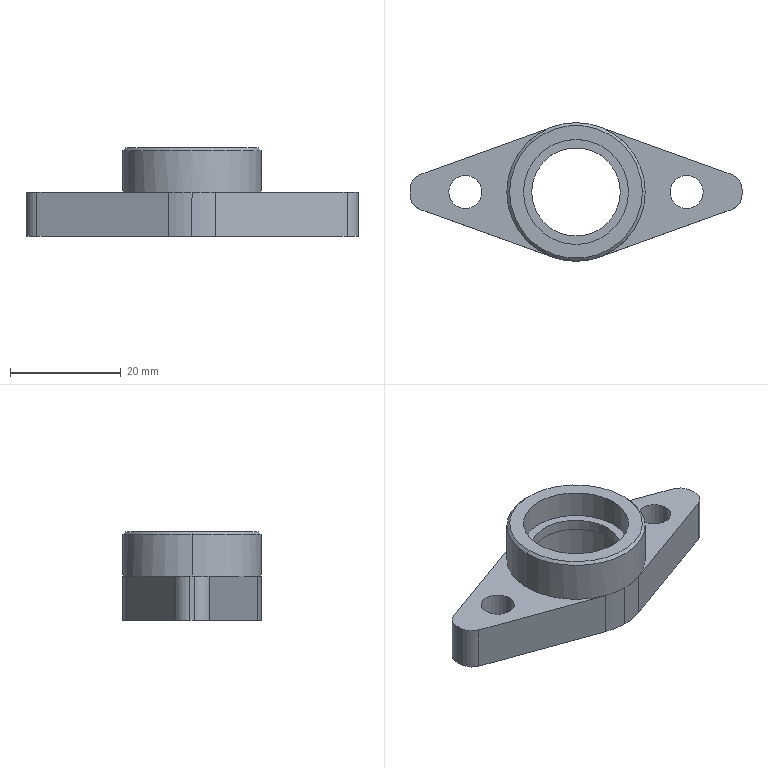Part | SolidWorks | features ICE 5, Fillet 2, MirrorPattern 2, Chamfer 1, Extrusion 1, HoleWzd 1 | 1 solid | 34 faces | box 60 x 25 x 16 mm | volume 6607 mm3 | cylinder 20 | plane 12 | cone 2 | commonest cylinder face diameters 6 x8 25 x6 19 x4 16 x2
STEP:
#1=CARTESIAN_POINT('',(-9.5,12.5,11.));
#2=VERTEX_POINT('',#1);
#3=CARTESIAN_POINT('',(9.5,12.5,11.));
#4=VERTEX_POINT('',#3);
#5=CARTESIAN_POINT('',(0.,12.5,11.));
#6=DIRECTION('',(0.,0.,1.));
#7=DIRECTION('',(1.,0.,0.));
#8=AXIS2_PLACEMENT_3D('',#5,#6,#7);
#9=CIRCLE('',#8,9.5);
#10=EDGE_CURVE('',#2,#4,#9,.T.);
#11=ORIENTED_EDGE('',*,*,#10,.F.);
#12=CARTESIAN_POINT('',(-9.5,12.5,16.));
#13=VERTEX_POINT('',#12);
#14=CARTESIAN_POINT('',(-9.5,12.5,11.));
#15=DIRECTION('',(0.,0.,1.));
#16=VECTOR('',#15,1000.);
#17=LINE('',#14,#16);
#18=EDGE_CURVE('',#2,#13,#17,.T.);
#19=ORIENTED_EDGE('',*,*,#18,.T.);
#20=CARTESIAN_POINT('',(9.5,12.5,16.));
#21=VERTEX_POINT('',#20);
#22=CARTESIAN_POINT('',(0.,12.5,16.));
#23=DIRECTION('',(0.,0.,1.));
#24=DIRECTION('',(1.,0.,0.));
#25=AXIS2_PLACEMENT_3D('',#22,#23,#24);
#26=CIRCLE('',#25,9.5);
#27=EDGE_CURVE('',#13,#21,#26,.T.);
#28=ORIENTED_EDGE('',*,*,#27,.T.);
#29=CARTESIAN_POINT('',(9.5,12.5,11.));
#30=DIRECTION('',(0.,0.,1.));
#31=VECTOR('',#30,1000.);
#32=LINE('',#29,#31);
#33=EDGE_CURVE('',#4,#21,#32,.T.);
#34=ORIENTED_EDGE('',*,*,#33,.F.);
#35=EDGE_LOOP('',(#11,#19,#28,#34));
#36=FACE_OUTER_BOUND('',#35,.T.);
#37=CARTESIAN_POINT('',(0.,12.5,11.));
#38=DIRECTION('',(0.,0.,1.));
#39=DIRECTION('',(1.,0.,0.));
#40=AXIS2_PLACEMENT_3D('',#37,#38,#39);
#41=CYLINDRICAL_SURFACE('',#40,9.5);
#42=ADVANCED_FACE('',(#36),#41,.F.);
#43=CARTESIAN_POINT('',(12.,12.5,16.));
#44=VERTEX_POINT('',#43);
#45=CARTESIAN_POINT('',(-12.,12.5,16.));
#46=VERTEX_POINT('',#45);
#47=CARTESIAN_POINT('',(0.,12.5,16.));
#48=DIRECTION('',(0.,0.,1.));
#49=DIRECTION('',(1.,0.,0.));
#50=AXIS2_PLACEMENT_3D('',#47,#48,#49);
#51=CIRCLE('',#50,12.);
#52=EDGE_CURVE('',#44,#46,#51,.T.);
#53=ORIENTED_EDGE('',*,*,#52,.F.);
#54=CARTESIAN_POINT('',(12.5,12.5,15.5));
#55=VERTEX_POINT('',#54);
#56=CARTESIAN_POINT('',(12.,12.5,16.));
#57=DIRECTION('',(0.7071,0.,-0.7071));
#58=VECTOR('',#57,1000.);
#59=LINE('',#56,#58);
#60=EDGE_CURVE('',#44,#55,#59,.T.);
#61=ORIENTED_EDGE('',*,*,#60,.T.);
#62=CARTESIAN_POINT('',(-12.5,12.5,15.5));
#63=VERTEX_POINT('',#62);
#64=CARTESIAN_POINT('',(0.,12.5,15.5));
#65=DIRECTION('',(0.,0.,-1.));
#66=DIRECTION('',(1.,0.,0.));
#67=AXIS2_PLACEMENT_3D('',#64,#65,#66);
#68=CIRCLE('',#67,12.5);
#69=EDGE_CURVE('',#63,#55,#68,.T.);
#70=ORIENTED_EDGE('',*,*,#69,.F.);
#71=CARTESIAN_POINT('',(-12.,12.5,16.));
#72=DIRECTION('',(-0.7071,0.,-0.7071));
#73=VECTOR('',#72,1000.);
#74=LINE('',#71,#73);
#75=EDGE_CURVE('',#46,#63,#74,.T.);
#76=ORIENTED_EDGE('',*,*,#75,.F.);
#77=EDGE_LOOP('',(#53,#61,#70,#76));
#78=FACE_OUTER_BOUND('',#77,.T.);
#79=CARTESIAN_POINT('',(0.,12.5,16.));
#80=DIRECTION('',(0.,0.,-1.));
#81=DIRECTION('',(-1.,0.,0.));
#82=AXIS2_PLACEMENT_3D('',#79,#80,#81);
#83=CONICAL_SURFACE('',#82,12.,0.7854);
#84=ADVANCED_FACE('',(#78),#83,.T.);
#85=CARTESIAN_POINT('',(17.,12.5,0.));
#86=VERTEX_POINT('',#85);
#87=CARTESIAN_POINT('',(23.,12.5,0.));
#88=VERTEX_POINT('',#87);
#89=CARTESIAN_POINT('',(20.,12.5,0.));
#90=DIRECTION('',(0.,0.,1.));
#91=DIRECTION('',(1.,0.,0.));
#92=AXIS2_PLACEMENT_3D('',#89,#90,#91);
#93=CIRCLE('',#92,3.);
#94=EDGE_CURVE('',#86,#88,#93,.T.);
#95=ORIENTED_EDGE('',*,*,#94,.F.);
#96=CARTESIAN_POINT('',(17.,12.5,8.));
#97=VERTEX_POINT('',#96);
#98=CARTESIAN_POINT('',(17.,12.5,8.));
#99=DIRECTION('',(0.,0.,1.));
#100=VECTOR('',#99,1000.);
#101=LINE('',#98,#100);
#102=EDGE_CURVE('',#86,#97,#101,.T.);
#103=ORIENTED_EDGE('',*,*,#102,.T.);
#104=CARTESIAN_POINT('',(23.,12.5,8.));
#105=VERTEX_POINT('',#104);
#106=CARTESIAN_POINT('',(20.,12.5,8.));
#107=DIRECTION('',(0.,0.,1.));
#108=DIRECTION('',(1.,0.,0.));
#109=AXIS2_PLACEMENT_3D('',#106,#107,#108);
#110=CIRCLE('',#109,3.);
#111=EDGE_CURVE('',#97,#105,#110,.T.);
#112=ORIENTED_EDGE('',*,*,#111,.T.);
#113=CARTESIAN_POINT('',(23.,12.5,8.));
#114=DIRECTION('',(0.,0.,1.));
#115=VECTOR('',#114,1000.);
#116=LINE('',#113,#115);
#117=EDGE_CURVE('',#88,#105,#116,.T.);
#118=ORIENTED_EDGE('',*,*,#117,.F.);
#119=EDGE_LOOP('',(#95,#103,#112,#118));
#120=FACE_OUTER_BOUND('',#119,.T.);
#121=CARTESIAN_POINT('',(20.,12.5,8.));
#122=DIRECTION('',(0.,0.,1.));
#123=DIRECTION('',(1.,0.,0.));
#124=AXIS2_PLACEMENT_3D('',#121,#122,#123);
#125=CYLINDRICAL_SURFACE('',#124,3.);
#126=ADVANCED_FACE('',(#120),#125,.F.);
#127=CARTESIAN_POINT('',(-23.,12.5,0.));
#128=VERTEX_POINT('',#127);
#129=CARTESIAN_POINT('',(-17.,12.5,0.));
#130=VERTEX_POINT('',#129);
#131=CARTESIAN_POINT('',(-20.,12.5,0.));
#132=DIRECTION('',(0.,0.,1.));
#133=DIRECTION('',(1.,0.,0.));
#134=AXIS2_PLACEMENT_3D('',#131,#132,#133);
#135=CIRCLE('',#134,3.);
#136=EDGE_CURVE('',#128,#130,#135,.T.);
#137=ORIENTED_EDGE('',*,*,#136,.F.);
#138=CARTESIAN_POINT('',(-23.,12.5,8.));
#139=VERTEX_POINT('',#138);
#140=CARTESIAN_POINT('',(-23.,12.5,8.));
#141=DIRECTION('',(0.,0.,1.));
#142=VECTOR('',#141,1000.);
#143=LINE('',#140,#142);
#144=EDGE_CURVE('',#128,#139,#143,.T.);
#145=ORIENTED_EDGE('',*,*,#144,.T.);
#146=CARTESIAN_POINT('',(-17.,12.5,8.));
#147=VERTEX_POINT('',#146);
#148=CARTESIAN_POINT('',(-20.,12.5,8.));
#149=DIRECTION('',(0.,0.,1.));
#150=DIRECTION('',(1.,0.,0.));
#151=AXIS2_PLACEMENT_3D('',#148,#149,#150);
#152=CIRCLE('',#151,3.);
#153=EDGE_CURVE('',#139,#147,#152,.T.);
#154=ORIENTED_EDGE('',*,*,#153,.T.);
#155=CARTESIAN_POINT('',(-17.,12.5,8.));
#156=DIRECTION('',(0.,0.,1.));
#157=VECTOR('',#156,1000.);
#158=LINE('',#155,#157);
#159=EDGE_CURVE('',#130,#147,#158,.T.);
#160=ORIENTED_EDGE('',*,*,#159,.F.);
#161=EDGE_LOOP('',(#137,#145,#154,#160));
#162=FACE_OUTER_BOUND('',#161,.T.);
#163=CARTESIAN_POINT('',(-20.,12.5,8.));
#164=DIRECTION('',(0.,0.,1.));
#165=DIRECTION('',(1.,0.,0.));
#166=AXIS2_PLACEMENT_3D('',#163,#164,#165);
#167=CYLINDRICAL_SURFACE('',#166,3.);
#168=ADVANCED_FACE('',(#162),#167,.F.);
#169=CARTESIAN_POINT('',(9.5,12.5,9.));
#170=VERTEX_POINT('',#169);
#171=CARTESIAN_POINT('',(-9.5,12.5,9.));
#172=VERTEX_POINT('',#171);
#173=CARTESIAN_POINT('',(0.,12.5,9.));
#174=DIRECTION('',(0.,0.,-1.));
#175=DIRECTION('',(-1.,0.,0.));
#176=AXIS2_PLACEMENT_3D('',#173,#174,#175);
#177=CIRCLE('',#176,9.5);
#178=EDGE_CURVE('',#170,#172,#177,.T.);
#179=ORIENTED_EDGE('',*,*,#178,.F.);
#180=CARTESIAN_POINT('',(9.5,12.5,0.));
#181=VERTEX_POINT('',#180);
#182=CARTESIAN_POINT('',(9.5,12.5,9.));
#183=DIRECTION('',(0.,0.,-1.));
#184=VECTOR('',#183,1000.);
#185=LINE('',#182,#184);
#186=EDGE_CURVE('',#170,#181,#185,.T.);
#187=ORIENTED_EDGE('',*,*,#186,.T.);
#188=CARTESIAN_POINT('',(-9.5,12.5,0.));
#189=VERTEX_POINT('',#188);
#190=CARTESIAN_POINT('',(0.,12.5,0.));
#191=DIRECTION('',(0.,0.,-1.));
#192=DIRECTION('',(-1.,0.,0.));
#193=AXIS2_PLACEMENT_3D('',#190,#191,#192);
#194=CIRCLE('',#193,9.5);
#195=EDGE_CURVE('',#181,#189,#194,.T.);
#196=ORIENTED_EDGE('',*,*,#195,.T.);
#197=CARTESIAN_POINT('',(-9.5,12.5,9.));
#198=DIRECTION('',(0.,0.,-1.));
#199=VECTOR('',#198,1000.);
#200=LINE('',#197,#199);
#201=EDGE_CURVE('',#172,#189,#200,.T.);
#202=ORIENTED_EDGE('',*,*,#201,.F.);
#203=EDGE_LOOP('',(#179,#187,#196,#202));
#204=FACE_OUTER_BOUND('',#203,.T.);
#205=CARTESIAN_POINT('',(0.,12.5,9.));
#206=DIRECTION('',(0.,0.,-1.));
#207=DIRECTION('',(-1.,0.,0.));
#208=AXIS2_PLACEMENT_3D('',#205,#206,#207);
#209=CYLINDRICAL_SURFACE('',#208,9.5);
#210=ADVANCED_FACE('',(#204),#209,.F.);
#211=ORIENTED_EDGE('',*,*,#69,.T.);
#212=CARTESIAN_POINT('',(12.5,12.5,8.));
#213=VERTEX_POINT('',#212);
#214=CARTESIAN_POINT('',(12.5,12.5,16.));
#215=DIRECTION('',(0.,0.,-1.));
#216=VECTOR('',#215,1000.);
#217=LINE('',#214,#216);
#218=EDGE_CURVE('',#55,#213,#217,.T.);
#219=ORIENTED_EDGE('',*,*,#218,.T.);
#220=CARTESIAN_POINT('',(4.228,24.263,8.));
#221=VERTEX_POINT('',#220);
#222=CARTESIAN_POINT('',(0.,12.5,8.));
#223=DIRECTION('',(0.,0.,1.));
#224=DIRECTION('',(1.,0.,0.));
#225=AXIS2_PLACEMENT_3D('',#222,#223,#224);
#226=CIRCLE('',#225,12.5);
#227=EDGE_CURVE('',#213,#221,#226,.T.);
#228=ORIENTED_EDGE('',*,*,#227,.T.);
#229=CARTESIAN_POINT('',(0.,25.,8.));
#230=VERTEX_POINT('',#229);
#231=CARTESIAN_POINT('',(0.,12.5,8.));
#232=DIRECTION('',(0.,0.,1.));
#233=DIRECTION('',(1.,0.,0.));
#234=AXIS2_PLACEMENT_3D('',#231,#232,#233);
#235=CIRCLE('',#234,12.5);
#236=EDGE_CURVE('',#221,#230,#235,.T.);
#237=ORIENTED_EDGE('',*,*,#236,.T.);
#238=CARTESIAN_POINT('',(-4.228,24.263,8.));
#239=VERTEX_POINT('',#238);
#240=CARTESIAN_POINT('',(0.,12.5,8.));
#241=DIRECTION('',(0.,0.,1.));
#242=DIRECTION('',(1.,0.,0.));
#243=AXIS2_PLACEMENT_3D('',#240,#241,#242);
#244=CIRCLE('',#243,12.5);
#245=EDGE_CURVE('',#230,#239,#244,.T.);
#246=ORIENTED_EDGE('',*,*,#245,.T.);
#247=CARTESIAN_POINT('',(-12.5,12.5,8.));
#248=VERTEX_POINT('',#247);
#249=CARTESIAN_POINT('',(0.,12.5,8.));
#250=DIRECTION('',(0.,0.,1.));
#251=DIRECTION('',(1.,0.,0.));
#252=AXIS2_PLACEMENT_3D('',#249,#250,#251);
#253=CIRCLE('',#252,12.5);
#254=EDGE_CURVE('',#239,#248,#253,.T.);
#255=ORIENTED_EDGE('',*,*,#254,.T.);
#256=CARTESIAN_POINT('',(-12.5,12.5,16.));
#257=DIRECTION('',(0.,0.,-1.));
#258=VECTOR('',#257,1000.);
#259=LINE('',#256,#258);
#260=EDGE_CURVE('',#63,#248,#259,.T.);
#261=ORIENTED_EDGE('',*,*,#260,.F.);
#262=EDGE_LOOP('',(#211,#219,#228,#237,#246,#255,#261));
#263=FACE_OUTER_BOUND('',#262,.T.);
#264=CARTESIAN_POINT('',(0.,12.5,16.));
#265=DIRECTION('',(0.,0.,-1.));
#266=DIRECTION('',(-1.,0.,0.));
#267=AXIS2_PLACEMENT_3D('',#264,#265,#266);
#268=CYLINDRICAL_SURFACE('',#267,12.5);
#269=ADVANCED_FACE('',(#263),#268,.T.);
#270=CARTESIAN_POINT('',(8.,12.5,11.));
#271=VERTEX_POINT('',#270);
#272=CARTESIAN_POINT('',(-8.,12.5,11.));
#273=VERTEX_POINT('',#272);
#274=CARTESIAN_POINT('',(0.,12.5,11.));
#275=DIRECTION('',(0.,0.,-1.));
#276=DIRECTION('',(1.,0.,0.));
#277=AXIS2_PLACEMENT_3D('',#274,#275,#276);
#278=CIRCLE('',#277,8.);
#279=EDGE_CURVE('',#271,#273,#278,.T.);
#280=ORIENTED_EDGE('',*,*,#279,.F.);
#281=CARTESIAN_POINT('',(8.,12.5,9.));
#282=VERTEX_POINT('',#281);
#283=CARTESIAN_POINT('',(8.,12.5,23.));
#284=DIRECTION('',(0.,0.,-1.));
#285=VECTOR('',#284,1000.);
#286=LINE('',#283,#285);
#287=EDGE_CURVE('',#271,#282,#286,.T.);
#288=ORIENTED_EDGE('',*,*,#287,.T.);
#289=CARTESIAN_POINT('',(-8.,12.5,9.));
#290=VERTEX_POINT('',#289);
#291=CARTESIAN_POINT('',(0.,12.5,9.));
#292=DIRECTION('',(0.,0.,-1.));
#293=DIRECTION('',(-1.,0.,0.));
#294=AXIS2_PLACEMENT_3D('',#291,#292,#293);
#295=CIRCLE('',#294,8.);
#296=EDGE_CURVE('',#282,#290,#295,.T.);
#297=ORIENTED_EDGE('',*,*,#296,.T.);
#298=CARTESIAN_POINT('',(-8.,12.5,23.));
#299=DIRECTION('',(0.,0.,-1.));
#300=VECTOR('',#299,1000.);
#301=LINE('',#298,#300);
#302=EDGE_CURVE('',#273,#290,#301,.T.);
#303=ORIENTED_EDGE('',*,*,#302,.F.);
#304=EDGE_LOOP('',(#280,#288,#297,#303));
#305=FACE_OUTER_BOUND('',#304,.T.);
#306=CARTESIAN_POINT('',(0.,12.5,23.));
#307=DIRECTION('',(0.,0.,-1.));
#308=DIRECTION('',(-1.,0.,0.));
#309=AXIS2_PLACEMENT_3D('',#306,#307,#308);
#310=CYLINDRICAL_SURFACE('',#309,8.);
#311=ADVANCED_FACE('',(#305),#310,.F.);
#312=ORIENTED_EDGE('',*,*,#287,.F.);
#313=CARTESIAN_POINT('',(0.,12.5,11.));
#314=DIRECTION('',(0.,0.,-1.));
#315=DIRECTION('',(1.,0.,0.));
#316=AXIS2_PLACEMENT_3D('',#313,#314,#315);
#317=CIRCLE('',#316,8.);
#318=EDGE_CURVE('',#273,#271,#317,.T.);
#319=ORIENTED_EDGE('',*,*,#318,.F.);
#320=ORIENTED_EDGE('',*,*,#302,.T.);
#321=CARTESIAN_POINT('',(0.,12.5,9.));
#322=DIRECTION('',(0.,0.,-1.));
#323=DIRECTION('',(-1.,0.,0.));
#324=AXIS2_PLACEMENT_3D('',#321,#322,#323);
#325=CIRCLE('',#324,8.);
#326=EDGE_CURVE('',#290,#282,#325,.T.);
#327=ORIENTED_EDGE('',*,*,#326,.T.);
#328=EDGE_LOOP('',(#312,#319,#320,#327));
#329=FACE_OUTER_BOUND('',#328,.T.);
#330=CARTESIAN_POINT('',(0.,12.5,23.));
#331=DIRECTION('',(0.,0.,-1.));
#332=DIRECTION('',(-1.,0.,0.));
#333=AXIS2_PLACEMENT_3D('',#330,#331,#332);
#334=CYLINDRICAL_SURFACE('',#333,8.);
#335=ADVANCED_FACE('',(#329),#334,.F.);
#336=CARTESIAN_POINT('',(20.,12.5,0.));
#337=DIRECTION('',(0.,0.,1.));
#338=DIRECTION('',(1.,0.,0.));
#339=AXIS2_PLACEMENT_3D('',#336,#337,#338);
#340=CIRCLE('',#339,3.);
#341=EDGE_CURVE('',#88,#86,#340,.T.);
#342=ORIENTED_EDGE('',*,*,#341,.T.);
#343=ORIENTED_EDGE('',*,*,#94,.T.);
#344=EDGE_LOOP('',(#342,#343));
#345=FACE_BOUND('',#344,.T.);
#346=CARTESIAN_POINT('',(-20.,12.5,0.));
#347=DIRECTION('',(0.,0.,1.));
#348=DIRECTION('',(1.,0.,0.));
#349=AXIS2_PLACEMENT_3D('',#346,#347,#348);
#350=CIRCLE('',#349,3.);
#351=EDGE_CURVE('',#130,#128,#350,.T.);
#352=ORIENTED_EDGE('',*,*,#351,.T.);
#353=ORIENTED_EDGE('',*,*,#136,.T.);
#354=EDGE_LOOP('',(#352,#353));
#355=FACE_BOUND('',#354,.T.);
#356=CARTESIAN_POINT('',(0.,12.5,0.));
#357=DIRECTION('',(0.,0.,-1.));
#358=DIRECTION('',(-1.,0.,0.));
#359=AXIS2_PLACEMENT_3D('',#356,#357,#358);
#360=CIRCLE('',#359,9.5);
#361=EDGE_CURVE('',#189,#181,#360,.T.);
#362=ORIENTED_EDGE('',*,*,#361,.F.);
#363=ORIENTED_EDGE('',*,*,#195,.F.);
#364=EDGE_LOOP('',(#362,#363));
#365=FACE_BOUND('',#364,.T.);
#366=CARTESIAN_POINT('',(-30.,12.89,0.));
#367=VERTEX_POINT('',#366);
#368=CARTESIAN_POINT('',(-30.,12.11,0.));
#369=VERTEX_POINT('',#368);
#370=CARTESIAN_POINT('',(-30.,25.,0.));
#371=DIRECTION('',(0.,-1.,0.));
#372=VECTOR('',#371,1000.);
#373=LINE('',#370,#372);
#374=EDGE_CURVE('',#367,#369,#373,.T.);
#375=ORIENTED_EDGE('',*,*,#374,.F.);
#376=CARTESIAN_POINT('',(-28.015,15.714,0.));
#377=VERTEX_POINT('',#376);
#378=CARTESIAN_POINT('',(-27.,12.89,0.));
#379=DIRECTION('',(0.,0.,-1.));
#380=DIRECTION('',(1.,0.,0.));
#381=AXIS2_PLACEMENT_3D('',#378,#379,#380);
#382=CIRCLE('',#381,3.);
#383=EDGE_CURVE('',#367,#377,#382,.T.);
#384=ORIENTED_EDGE('',*,*,#383,.T.);
#385=CARTESIAN_POINT('',(-4.228,24.263,0.));
#386=VERTEX_POINT('',#385);
#387=CARTESIAN_POINT('',(-8.207,22.833,0.));
#388=DIRECTION('',(-0.9411,-0.3382,0.));
#389=VECTOR('',#388,1000.);
#390=LINE('',#387,#389);
#391=EDGE_CURVE('',#386,#377,#390,.T.);
#392=ORIENTED_EDGE('',*,*,#391,.F.);
#393=CARTESIAN_POINT('',(0.,25.,0.));
#394=VERTEX_POINT('',#393);
#395=CARTESIAN_POINT('',(0.,12.5,0.));
#396=DIRECTION('',(0.,0.,-1.));
#397=DIRECTION('',(1.,0.,0.));
#398=AXIS2_PLACEMENT_3D('',#395,#396,#397);
#399=CIRCLE('',#398,12.5);
#400=EDGE_CURVE('',#386,#394,#399,.T.);
#401=ORIENTED_EDGE('',*,*,#400,.T.);
#402=CARTESIAN_POINT('',(4.228,24.263,0.));
#403=VERTEX_POINT('',#402);
#404=CARTESIAN_POINT('',(0.,12.5,0.));
#405=DIRECTION('',(0.,0.,-1.));
#406=DIRECTION('',(1.,0.,0.));
#407=AXIS2_PLACEMENT_3D('',#404,#405,#406);
#408=CIRCLE('',#407,12.5);
#409=EDGE_CURVE('',#394,#403,#408,.T.);
#410=ORIENTED_EDGE('',*,*,#409,.T.);
#411=CARTESIAN_POINT('',(28.015,15.714,0.));
#412=VERTEX_POINT('',#411);
#413=CARTESIAN_POINT('',(8.207,22.833,0.));
#414=DIRECTION('',(0.9411,-0.3382,0.));
#415=VECTOR('',#414,1000.);
#416=LINE('',#413,#415);
#417=EDGE_CURVE('',#403,#412,#416,.T.);
#418=ORIENTED_EDGE('',*,*,#417,.T.);
#419=CARTESIAN_POINT('',(30.,12.89,0.));
#420=VERTEX_POINT('',#419);
#421=CARTESIAN_POINT('',(27.,12.89,0.));
#422=DIRECTION('',(0.,0.,-1.));
#423=DIRECTION('',(1.,0.,0.));
#424=AXIS2_PLACEMENT_3D('',#421,#422,#423);
#425=CIRCLE('',#424,3.);
#426=EDGE_CURVE('',#412,#420,#425,.T.);
#427=ORIENTED_EDGE('',*,*,#426,.T.);
#428=CARTESIAN_POINT('',(30.,12.11,0.));
#429=VERTEX_POINT('',#428);
#430=CARTESIAN_POINT('',(30.,25.,0.));
#431=DIRECTION('',(0.,1.,0.));
#432=VECTOR('',#431,1000.);
#433=LINE('',#430,#432);
#434=EDGE_CURVE('',#429,#420,#433,.T.);
#435=ORIENTED_EDGE('',*,*,#434,.F.);
#436=CARTESIAN_POINT('',(28.015,9.286,0.));
#437=VERTEX_POINT('',#436);
#438=CARTESIAN_POINT('',(27.,12.11,0.));
#439=DIRECTION('',(0.,0.,-1.));
#440=DIRECTION('',(1.,0.,0.));
#441=AXIS2_PLACEMENT_3D('',#438,#439,#440);
#442=CIRCLE('',#441,3.);
#443=EDGE_CURVE('',#429,#437,#442,.T.);
#444=ORIENTED_EDGE('',*,*,#443,.T.);
#445=CARTESIAN_POINT('',(4.228,0.7368,0.));
#446=VERTEX_POINT('',#445);
#447=CARTESIAN_POINT('',(0.2492,-0.6933,0.));
#448=DIRECTION('',(0.9411,0.3382,0.));
#449=VECTOR('',#448,1000.);
#450=LINE('',#447,#449);
#451=EDGE_CURVE('',#446,#437,#450,.T.);
#452=ORIENTED_EDGE('',*,*,#451,.F.);
#453=CARTESIAN_POINT('',(0.,0.,0.));
#454=VERTEX_POINT('',#453);
#455=CARTESIAN_POINT('',(0.,12.5,0.));
#456=DIRECTION('',(0.,0.,-1.));
#457=DIRECTION('',(1.,0.,0.));
#458=AXIS2_PLACEMENT_3D('',#455,#456,#457);
#459=CIRCLE('',#458,12.5);
#460=EDGE_CURVE('',#446,#454,#459,.T.);
#461=ORIENTED_EDGE('',*,*,#460,.T.);
#462=CARTESIAN_POINT('',(-4.228,0.7368,0.));
#463=VERTEX_POINT('',#462);
#464=CARTESIAN_POINT('',(0.,12.5,0.));
#465=DIRECTION('',(0.,0.,-1.));
#466=DIRECTION('',(1.,0.,0.));
#467=AXIS2_PLACEMENT_3D('',#464,#465,#466);
#468=CIRCLE('',#467,12.5);
#469=EDGE_CURVE('',#454,#463,#468,.T.);
#470=ORIENTED_EDGE('',*,*,#469,.T.);
#471=CARTESIAN_POINT('',(-28.015,9.286,0.));
#472=VERTEX_POINT('',#471);
#473=CARTESIAN_POINT('',(-0.2492,-0.6933,0.));
#474=DIRECTION('',(-0.9411,0.3382,0.));
#475=VECTOR('',#474,1000.);
#476=LINE('',#473,#475);
#477=EDGE_CURVE('',#463,#472,#476,.T.);
#478=ORIENTED_EDGE('',*,*,#477,.T.);
#479=CARTESIAN_POINT('',(-27.,12.11,0.));
#480=DIRECTION('',(0.,0.,-1.));
#481=DIRECTION('',(1.,0.,0.));
#482=AXIS2_PLACEMENT_3D('',#479,#480,#481);
#483=CIRCLE('',#482,3.);
#484=EDGE_CURVE('',#472,#369,#483,.T.);
#485=ORIENTED_EDGE('',*,*,#484,.T.);
#486=EDGE_LOOP('',(#375,#384,#392,#401,#410,#418,#427,#435,#444,#452,#461,#470,#478,#485));
#487=FACE_OUTER_BOUND('',#486,.T.);
#488=CARTESIAN_POINT('',(0.,0.,0.));
#489=DIRECTION('',(0.,0.,1.));
#490=DIRECTION('',(1.,0.,0.));
#491=AXIS2_PLACEMENT_3D('',#488,#489,#490);
#492=PLANE('',#491);
#493=ADVANCED_FACE('',(#345,#355,#365,#487),#492,.F.);
#494=CARTESIAN_POINT('',(-20.,12.5,8.));
#495=DIRECTION('',(0.,0.,1.));
#496=DIRECTION('',(1.,0.,0.));
#497=AXIS2_PLACEMENT_3D('',#494,#495,#496);
#498=CIRCLE('',#497,3.);
#499=EDGE_CURVE('',#147,#139,#498,.T.);
#500=ORIENTED_EDGE('',*,*,#499,.F.);
#501=ORIENTED_EDGE('',*,*,#153,.F.);
#502=EDGE_LOOP('',(#500,#501));
#503=FACE_BOUND('',#502,.T.);
#504=CARTESIAN_POINT('',(-28.015,15.714,8.));
#505=VERTEX_POINT('',#504);
#506=CARTESIAN_POINT('',(-2.178,25.,8.));
#507=DIRECTION('',(-0.9411,-0.3382,0.));
#508=VECTOR('',#507,1000.);
#509=LINE('',#506,#508);
#510=EDGE_CURVE('',#239,#505,#509,.T.);
#511=ORIENTED_EDGE('',*,*,#510,.T.);
#512=CARTESIAN_POINT('',(-30.,12.89,8.));
#513=VERTEX_POINT('',#512);
#514=CARTESIAN_POINT('',(-27.,12.89,8.));
#515=DIRECTION('',(0.,0.,1.));
#516=DIRECTION('',(1.,0.,0.));
#517=AXIS2_PLACEMENT_3D('',#514,#515,#516);
#518=CIRCLE('',#517,3.);
#519=EDGE_CURVE('',#505,#513,#518,.T.);
#520=ORIENTED_EDGE('',*,*,#519,.T.);
#521=CARTESIAN_POINT('',(-30.,12.11,8.));
#522=VERTEX_POINT('',#521);
#523=CARTESIAN_POINT('',(-30.,25.,8.));
#524=DIRECTION('',(0.,-1.,0.));
#525=VECTOR('',#524,1000.);
#526=LINE('',#523,#525);
#527=EDGE_CURVE('',#513,#522,#526,.T.);
#528=ORIENTED_EDGE('',*,*,#527,.T.);
#529=CARTESIAN_POINT('',(-28.015,9.286,8.));
#530=VERTEX_POINT('',#529);
#531=CARTESIAN_POINT('',(-27.,12.11,8.));
#532=DIRECTION('',(0.,0.,1.));
#533=DIRECTION('',(1.,0.,0.));
#534=AXIS2_PLACEMENT_3D('',#531,#532,#533);
#535=CIRCLE('',#534,3.);
#536=EDGE_CURVE('',#522,#530,#535,.T.);
#537=ORIENTED_EDGE('',*,*,#536,.T.);
#538=CARTESIAN_POINT('',(-4.228,0.7368,8.));
#539=VERTEX_POINT('',#538);
#540=CARTESIAN_POINT('',(-2.178,0.,8.));
#541=DIRECTION('',(-0.9411,0.3382,0.));
#542=VECTOR('',#541,1000.);
#543=LINE('',#540,#542);
#544=EDGE_CURVE('',#539,#530,#543,.T.);
#545=ORIENTED_EDGE('',*,*,#544,.F.);
#546=CARTESIAN_POINT('',(0.,12.5,8.));
#547=DIRECTION('',(0.,0.,1.));
#548=DIRECTION('',(1.,0.,0.));
#549=AXIS2_PLACEMENT_3D('',#546,#547,#548);
#550=CIRCLE('',#549,12.5);
#551=EDGE_CURVE('',#248,#539,#550,.T.);
#552=ORIENTED_EDGE('',*,*,#551,.F.);
#553=ORIENTED_EDGE('',*,*,#254,.F.);
#554=EDGE_LOOP('',(#511,#520,#528,#537,#545,#552,#553));
#555=FACE_OUTER_BOUND('',#554,.T.);
#556=CARTESIAN_POINT('',(0.,0.,8.));
#557=DIRECTION('',(0.,0.,1.));
#558=DIRECTION('',(1.,0.,0.));
#559=AXIS2_PLACEMENT_3D('',#556,#557,#558);
#560=PLANE('',#559);
#561=ADVANCED_FACE('',(#503,#555),#560,.T.);
#562=ORIENTED_EDGE('',*,*,#527,.F.);
#563=CARTESIAN_POINT('',(-30.,12.89,0.));
#564=DIRECTION('',(0.,0.,-1.));
#565=VECTOR('',#564,1000.);
#566=LINE('',#563,#565);
#567=EDGE_CURVE('',#513,#367,#566,.T.);
#568=ORIENTED_EDGE('',*,*,#567,.T.);
#569=ORIENTED_EDGE('',*,*,#374,.T.);
#570=CARTESIAN_POINT('',(-30.,12.11,8.));
#571=DIRECTION('',(0.,0.,1.));
#572=VECTOR('',#571,1000.);
#573=LINE('',#570,#572);
#574=EDGE_CURVE('',#369,#522,#573,.T.);
#575=ORIENTED_EDGE('',*,*,#574,.T.);
#576=EDGE_LOOP('',(#562,#568,#569,#575));
#577=FACE_OUTER_BOUND('',#576,.T.);
#578=CARTESIAN_POINT('',(-30.,25.,8.));
#579=DIRECTION('',(1.,0.,0.));
#580=DIRECTION('',(0.,1.,0.));
#581=AXIS2_PLACEMENT_3D('',#578,#579,#580);
#582=PLANE('',#581);
#583=ADVANCED_FACE('',(#577),#582,.F.);
#584=ORIENTED_EDGE('',*,*,#434,.T.);
#585=CARTESIAN_POINT('',(30.,12.89,8.));
#586=VERTEX_POINT('',#585);
#587=CARTESIAN_POINT('',(30.,12.89,8.));
#588=DIRECTION('',(0.,0.,1.));
#589=VECTOR('',#588,1000.);
#590=LINE('',#587,#589);
#591=EDGE_CURVE('',#420,#586,#590,.T.);
#592=ORIENTED_EDGE('',*,*,#591,.T.);
#593=CARTESIAN_POINT('',(30.,12.11,8.));
#594=VERTEX_POINT('',#593);
#595=CARTESIAN_POINT('',(30.,25.,8.));
#596=DIRECTION('',(0.,1.,0.));
#597=VECTOR('',#596,1000.);
#598=LINE('',#595,#597);
#599=EDGE_CURVE('',#594,#586,#598,.T.);
#600=ORIENTED_EDGE('',*,*,#599,.F.);
#601=CARTESIAN_POINT('',(30.,12.11,0.));
#602=DIRECTION('',(0.,0.,-1.));
#603=VECTOR('',#602,1000.);
#604=LINE('',#601,#603);
#605=EDGE_CURVE('',#594,#429,#604,.T.);
#606=ORIENTED_EDGE('',*,*,#605,.T.);
#607=EDGE_LOOP('',(#584,#592,#600,#606));
#608=FACE_OUTER_BOUND('',#607,.T.);
#609=CARTESIAN_POINT('',(30.,25.,8.));
#610=DIRECTION('',(-1.,0.,0.));
#611=DIRECTION('',(0.,-1.,0.));
#612=AXIS2_PLACEMENT_3D('',#609,#610,#611);
#613=PLANE('',#612);
#614=ADVANCED_FACE('',(#608),#613,.F.);
#615=CARTESIAN_POINT('',(20.,12.5,8.));
#616=DIRECTION('',(0.,0.,1.));
#617=DIRECTION('',(1.,0.,0.));
#618=AXIS2_PLACEMENT_3D('',#615,#616,#617);
#619=CIRCLE('',#618,3.);
#620=EDGE_CURVE('',#105,#97,#619,.T.);
#621=ORIENTED_EDGE('',*,*,#620,.F.);
#622=ORIENTED_EDGE('',*,*,#111,.F.);
#623=EDGE_LOOP('',(#621,#622));
#624=FACE_BOUND('',#623,.T.);
#625=ORIENTED_EDGE('',*,*,#599,.T.);
#626=CARTESIAN_POINT('',(28.015,15.714,8.));
#627=VERTEX_POINT('',#626);
#628=CARTESIAN_POINT('',(27.,12.89,8.));
#629=DIRECTION('',(0.,0.,1.));
#630=DIRECTION('',(1.,0.,0.));
#631=AXIS2_PLACEMENT_3D('',#628,#629,#630);
#632=CIRCLE('',#631,3.);
#633=EDGE_CURVE('',#586,#627,#632,.T.);
#634=ORIENTED_EDGE('',*,*,#633,.T.);
#635=CARTESIAN_POINT('',(2.178,25.,8.));
#636=DIRECTION('',(0.9411,-0.3382,0.));
#637=VECTOR('',#636,1000.);
#638=LINE('',#635,#637);
#639=EDGE_CURVE('',#221,#627,#638,.T.);
#640=ORIENTED_EDGE('',*,*,#639,.F.);
#641=ORIENTED_EDGE('',*,*,#227,.F.);
#642=CARTESIAN_POINT('',(4.228,0.7368,8.));
#643=VERTEX_POINT('',#642);
#644=CARTESIAN_POINT('',(0.,12.5,8.));
#645=DIRECTION('',(0.,0.,1.));
#646=DIRECTION('',(1.,0.,0.));
#647=AXIS2_PLACEMENT_3D('',#644,#645,#646);
#648=CIRCLE('',#647,12.5);
#649=EDGE_CURVE('',#643,#213,#648,.T.);
#650=ORIENTED_EDGE('',*,*,#649,.F.);
#651=CARTESIAN_POINT('',(28.015,9.286,8.));
#652=VERTEX_POINT('',#651);
#653=CARTESIAN_POINT('',(2.178,0.,8.));
#654=DIRECTION('',(0.9411,0.3382,0.));
#655=VECTOR('',#654,1000.);
#656=LINE('',#653,#655);
#657=EDGE_CURVE('',#643,#652,#656,.T.);
#658=ORIENTED_EDGE('',*,*,#657,.T.);
#659=CARTESIAN_POINT('',(27.,12.11,8.));
#660=DIRECTION('',(0.,0.,1.));
#661=DIRECTION('',(1.,0.,0.));
#662=AXIS2_PLACEMENT_3D('',#659,#660,#661);
#663=CIRCLE('',#662,3.);
#664=EDGE_CURVE('',#652,#594,#663,.T.);
#665=ORIENTED_EDGE('',*,*,#664,.T.);
#666=EDGE_LOOP('',(#625,#634,#640,#641,#650,#658,#665));
#667=FACE_OUTER_BOUND('',#666,.T.);
#668=CARTESIAN_POINT('',(0.,0.,8.));
#669=DIRECTION('',(0.,0.,1.));
#670=DIRECTION('',(1.,0.,0.));
#671=AXIS2_PLACEMENT_3D('',#668,#669,#670);
#672=PLANE('',#671);
#673=ADVANCED_FACE('',(#624,#667),#672,.T.);
#674=ORIENTED_EDGE('',*,*,#218,.F.);
#675=CARTESIAN_POINT('',(0.,12.5,15.5));
#676=DIRECTION('',(0.,0.,-1.));
#677=DIRECTION('',(1.,0.,0.));
#678=AXIS2_PLACEMENT_3D('',#675,#676,#677);
#679=CIRCLE('',#678,12.5);
#680=EDGE_CURVE('',#55,#63,#679,.T.);
#681=ORIENTED_EDGE('',*,*,#680,.T.);
#682=ORIENTED_EDGE('',*,*,#260,.T.);
#683=ORIENTED_EDGE('',*,*,#551,.T.);
#684=CARTESIAN_POINT('',(0.,0.,8.));
#685=VERTEX_POINT('',#684);
#686=CARTESIAN_POINT('',(0.,12.5,8.));
#687=DIRECTION('',(0.,0.,1.));
#688=DIRECTION('',(1.,0.,0.));
#689=AXIS2_PLACEMENT_3D('',#686,#687,#688);
#690=CIRCLE('',#689,12.5);
#691=EDGE_CURVE('',#539,#685,#690,.T.);
#692=ORIENTED_EDGE('',*,*,#691,.T.);
#693=CARTESIAN_POINT('',(0.,12.5,8.));
#694=DIRECTION('',(0.,0.,1.));
#695=DIRECTION('',(1.,0.,0.));
#696=AXIS2_PLACEMENT_3D('',#693,#694,#695);
#697=CIRCLE('',#696,12.5);
#698=EDGE_CURVE('',#685,#643,#697,.T.);
#699=ORIENTED_EDGE('',*,*,#698,.T.);
#700=ORIENTED_EDGE('',*,*,#649,.T.);
#701=EDGE_LOOP('',(#674,#681,#682,#683,#692,#699,#700));
#702=FACE_OUTER_BOUND('',#701,.T.);
#703=CARTESIAN_POINT('',(0.,12.5,16.));
#704=DIRECTION('',(0.,0.,-1.));
#705=DIRECTION('',(-1.,0.,0.));
#706=AXIS2_PLACEMENT_3D('',#703,#704,#705);
#707=CYLINDRICAL_SURFACE('',#706,12.5);
#708=ADVANCED_FACE('',(#702),#707,.T.);
#709=CARTESIAN_POINT('',(0.,12.5,16.));
#710=DIRECTION('',(0.,0.,1.));
#711=DIRECTION('',(1.,0.,0.));
#712=AXIS2_PLACEMENT_3D('',#709,#710,#711);
#713=CIRCLE('',#712,9.5);
#714=EDGE_CURVE('',#21,#13,#713,.T.);
#715=ORIENTED_EDGE('',*,*,#714,.F.);
#716=ORIENTED_EDGE('',*,*,#27,.F.);
#717=EDGE_LOOP('',(#715,#716));
#718=FACE_BOUND('',#717,.T.);
#719=CARTESIAN_POINT('',(0.,12.5,16.));
#720=DIRECTION('',(0.,0.,1.));
#721=DIRECTION('',(1.,0.,0.));
#722=AXIS2_PLACEMENT_3D('',#719,#720,#721);
#723=CIRCLE('',#722,12.);
#724=EDGE_CURVE('',#46,#44,#723,.T.);
#725=ORIENTED_EDGE('',*,*,#724,.T.);
#726=ORIENTED_EDGE('',*,*,#52,.T.);
#727=EDGE_LOOP('',(#725,#726));
#728=FACE_OUTER_BOUND('',#727,.T.);
#729=CARTESIAN_POINT('',(0.,12.5,16.));
#730=DIRECTION('',(0.,0.,1.));
#731=DIRECTION('',(1.,0.,0.));
#732=AXIS2_PLACEMENT_3D('',#729,#730,#731);
#733=PLANE('',#732);
#734=ADVANCED_FACE('',(#718,#728),#733,.T.);
#735=ORIENTED_EDGE('',*,*,#186,.F.);
#736=CARTESIAN_POINT('',(0.,12.5,9.));
#737=DIRECTION('',(0.,0.,-1.));
#738=DIRECTION('',(-1.,0.,0.));
#739=AXIS2_PLACEMENT_3D('',#736,#737,#738);
#740=CIRCLE('',#739,9.5);
#741=EDGE_CURVE('',#172,#170,#740,.T.);
#742=ORIENTED_EDGE('',*,*,#741,.F.);
#743=ORIENTED_EDGE('',*,*,#201,.T.);
#744=ORIENTED_EDGE('',*,*,#361,.T.);
#745=EDGE_LOOP('',(#735,#742,#743,#744));
#746=FACE_OUTER_BOUND('',#745,.T.);
#747=CARTESIAN_POINT('',(0.,12.5,9.));
#748=DIRECTION('',(0.,0.,-1.));
#749=DIRECTION('',(-1.,0.,0.));
#750=AXIS2_PLACEMENT_3D('',#747,#748,#749);
#751=CYLINDRICAL_SURFACE('',#750,9.5);
#752=ADVANCED_FACE('',(#746),#751,.F.);
#753=ORIENTED_EDGE('',*,*,#326,.F.);
#754=ORIENTED_EDGE('',*,*,#296,.F.);
#755=EDGE_LOOP('',(#753,#754));
#756=FACE_BOUND('',#755,.T.);
#757=ORIENTED_EDGE('',*,*,#741,.T.);
#758=ORIENTED_EDGE('',*,*,#178,.T.);
#759=EDGE_LOOP('',(#757,#758));
#760=FACE_OUTER_BOUND('',#759,.T.);
#761=CARTESIAN_POINT('',(0.,12.5,9.));
#762=DIRECTION('',(0.,0.,-1.));
#763=DIRECTION('',(-1.,0.,0.));
#764=AXIS2_PLACEMENT_3D('',#761,#762,#763);
#765=PLANE('',#764);
#766=ADVANCED_FACE('',(#756,#760),#765,.T.);
#767=ORIENTED_EDGE('',*,*,#144,.F.);
#768=ORIENTED_EDGE('',*,*,#351,.F.);
#769=ORIENTED_EDGE('',*,*,#159,.T.);
#770=ORIENTED_EDGE('',*,*,#499,.T.);
#771=EDGE_LOOP('',(#767,#768,#769,#770));
#772=FACE_OUTER_BOUND('',#771,.T.);
#773=CARTESIAN_POINT('',(-20.,12.5,8.));
#774=DIRECTION('',(0.,0.,1.));
#775=DIRECTION('',(1.,0.,0.));
#776=AXIS2_PLACEMENT_3D('',#773,#774,#775);
#777=CYLINDRICAL_SURFACE('',#776,3.);
#778=ADVANCED_FACE('',(#772),#777,.F.);
#779=ORIENTED_EDGE('',*,*,#102,.F.);
#780=ORIENTED_EDGE('',*,*,#341,.F.);
#781=ORIENTED_EDGE('',*,*,#117,.T.);
#782=ORIENTED_EDGE('',*,*,#620,.T.);
#783=EDGE_LOOP('',(#779,#780,#781,#782));
#784=FACE_OUTER_BOUND('',#783,.T.);
#785=CARTESIAN_POINT('',(20.,12.5,8.));
#786=DIRECTION('',(0.,0.,1.));
#787=DIRECTION('',(1.,0.,0.));
#788=AXIS2_PLACEMENT_3D('',#785,#786,#787);
#789=CYLINDRICAL_SURFACE('',#788,3.);
#790=ADVANCED_FACE('',(#784),#789,.F.);
#791=ORIENTED_EDGE('',*,*,#639,.T.);
#792=CARTESIAN_POINT('',(28.015,15.714,-5.));
#793=DIRECTION('',(0.,0.,-1.));
#794=VECTOR('',#793,1000.);
#795=LINE('',#792,#794);
#796=EDGE_CURVE('',#627,#412,#795,.T.);
#797=ORIENTED_EDGE('',*,*,#796,.T.);
#798=ORIENTED_EDGE('',*,*,#417,.F.);
#799=CARTESIAN_POINT('',(4.228,24.263,-5.));
#800=DIRECTION('',(0.,0.,1.));
#801=VECTOR('',#800,1000.);
#802=LINE('',#799,#801);
#803=EDGE_CURVE('',#403,#221,#802,.T.);
#804=ORIENTED_EDGE('',*,*,#803,.T.);
#805=EDGE_LOOP('',(#791,#797,#798,#804));
#806=FACE_OUTER_BOUND('',#805,.T.);
#807=CARTESIAN_POINT('',(2.178,25.,-5.));
#808=DIRECTION('',(-0.3382,-0.9411,0.));
#809=DIRECTION('',(0.9411,-0.3382,0.));
#810=AXIS2_PLACEMENT_3D('',#807,#808,#809);
#811=PLANE('',#810);
#812=ADVANCED_FACE('',(#806),#811,.F.);
#813=ORIENTED_EDGE('',*,*,#451,.T.);
#814=CARTESIAN_POINT('',(28.015,9.286,8.));
#815=DIRECTION('',(0.,0.,1.));
#816=VECTOR('',#815,1000.);
#817=LINE('',#814,#816);
#818=EDGE_CURVE('',#437,#652,#817,.T.);
#819=ORIENTED_EDGE('',*,*,#818,.T.);
#820=ORIENTED_EDGE('',*,*,#657,.F.);
#821=CARTESIAN_POINT('',(4.228,0.7368,0.));
#822=DIRECTION('',(0.,0.,-1.));
#823=VECTOR('',#822,1000.);
#824=LINE('',#821,#823);
#825=EDGE_CURVE('',#643,#446,#824,.T.);
#826=ORIENTED_EDGE('',*,*,#825,.T.);
#827=EDGE_LOOP('',(#813,#819,#820,#826));
#828=FACE_OUTER_BOUND('',#827,.T.);
#829=CARTESIAN_POINT('',(2.178,0.,-5.));
#830=DIRECTION('',(0.3382,-0.9411,0.));
#831=DIRECTION('',(0.9411,0.3382,0.));
#832=AXIS2_PLACEMENT_3D('',#829,#830,#831);
#833=PLANE('',#832);
#834=ADVANCED_FACE('',(#828),#833,.T.);
#835=ORIENTED_EDGE('',*,*,#544,.T.);
#836=CARTESIAN_POINT('',(-28.015,9.286,-5.));
#837=DIRECTION('',(0.,0.,-1.));
#838=VECTOR('',#837,1000.);
#839=LINE('',#836,#838);
#840=EDGE_CURVE('',#530,#472,#839,.T.);
#841=ORIENTED_EDGE('',*,*,#840,.T.);
#842=ORIENTED_EDGE('',*,*,#477,.F.);
#843=CARTESIAN_POINT('',(-4.228,0.7368,-5.));
#844=DIRECTION('',(0.,0.,1.));
#845=VECTOR('',#844,1000.);
#846=LINE('',#843,#845);
#847=EDGE_CURVE('',#463,#539,#846,.T.);
#848=ORIENTED_EDGE('',*,*,#847,.T.);
#849=EDGE_LOOP('',(#835,#841,#842,#848));
#850=FACE_OUTER_BOUND('',#849,.T.);
#851=CARTESIAN_POINT('',(-2.178,0.,-5.));
#852=DIRECTION('',(0.3382,0.9411,0.));
#853=DIRECTION('',(-0.9411,0.3382,0.));
#854=AXIS2_PLACEMENT_3D('',#851,#852,#853);
#855=PLANE('',#854);
#856=ADVANCED_FACE('',(#850),#855,.F.);
#857=ORIENTED_EDGE('',*,*,#391,.T.);
#858=CARTESIAN_POINT('',(-28.015,15.714,8.));
#859=DIRECTION('',(0.,0.,1.));
#860=VECTOR('',#859,1000.);
#861=LINE('',#858,#860);
#862=EDGE_CURVE('',#377,#505,#861,.T.);
#863=ORIENTED_EDGE('',*,*,#862,.T.);
#864=ORIENTED_EDGE('',*,*,#510,.F.);
#865=CARTESIAN_POINT('',(-4.228,24.263,0.));
#866=DIRECTION('',(0.,0.,-1.));
#867=VECTOR('',#866,1000.);
#868=LINE('',#865,#867);
#869=EDGE_CURVE('',#239,#386,#868,.T.);
#870=ORIENTED_EDGE('',*,*,#869,.T.);
#871=EDGE_LOOP('',(#857,#863,#864,#870));
#872=FACE_OUTER_BOUND('',#871,.T.);
#873=CARTESIAN_POINT('',(-2.178,25.,-5.));
#874=DIRECTION('',(-0.3382,0.9411,0.));
#875=DIRECTION('',(-0.9411,-0.3382,0.));
#876=AXIS2_PLACEMENT_3D('',#873,#874,#875);
#877=PLANE('',#876);
#878=ADVANCED_FACE('',(#872),#877,.T.);
#879=ORIENTED_EDGE('',*,*,#847,.F.);
#880=ORIENTED_EDGE('',*,*,#469,.F.);
#881=CARTESIAN_POINT('',(0.,0.,8.));
#882=DIRECTION('',(0.,0.,-1.));
#883=VECTOR('',#882,1000.);
#884=LINE('',#881,#883);
#885=EDGE_CURVE('',#685,#454,#884,.T.);
#886=ORIENTED_EDGE('',*,*,#885,.F.);
#887=ORIENTED_EDGE('',*,*,#691,.F.);
#888=EDGE_LOOP('',(#879,#880,#886,#887));
#889=FACE_OUTER_BOUND('',#888,.T.);
#890=CARTESIAN_POINT('',(0.,12.5,-5.));
#891=DIRECTION('',(0.,0.,1.));
#892=DIRECTION('',(1.,0.,0.));
#893=AXIS2_PLACEMENT_3D('',#890,#891,#892);
#894=CYLINDRICAL_SURFACE('',#893,12.5);
#895=ADVANCED_FACE('',(#889),#894,.T.);
#896=ORIENTED_EDGE('',*,*,#460,.F.);
#897=ORIENTED_EDGE('',*,*,#825,.F.);
#898=ORIENTED_EDGE('',*,*,#698,.F.);
#899=ORIENTED_EDGE('',*,*,#885,.T.);
#900=EDGE_LOOP('',(#896,#897,#898,#899));
#901=FACE_OUTER_BOUND('',#900,.T.);
#902=CARTESIAN_POINT('',(0.,12.5,8.));
#903=DIRECTION('',(0.,0.,-1.));
#904=DIRECTION('',(-1.,0.,0.));
#905=AXIS2_PLACEMENT_3D('',#902,#903,#904);
#906=CYLINDRICAL_SURFACE('',#905,12.5);
#907=ADVANCED_FACE('',(#901),#906,.T.);
#908=CARTESIAN_POINT('',(0.,25.,8.));
#909=DIRECTION('',(0.,0.,1.));
#910=VECTOR('',#909,1000.);
#911=LINE('',#908,#910);
#912=EDGE_CURVE('',#394,#230,#911,.T.);
#913=ORIENTED_EDGE('',*,*,#912,.F.);
#914=ORIENTED_EDGE('',*,*,#400,.F.);
#915=ORIENTED_EDGE('',*,*,#869,.F.);
#916=ORIENTED_EDGE('',*,*,#245,.F.);
#917=EDGE_LOOP('',(#913,#914,#915,#916));
#918=FACE_OUTER_BOUND('',#917,.T.);
#919=CARTESIAN_POINT('',(0.,12.5,-5.));
#920=DIRECTION('',(0.,0.,1.));
#921=DIRECTION('',(1.,0.,0.));
#922=AXIS2_PLACEMENT_3D('',#919,#920,#921);
#923=CYLINDRICAL_SURFACE('',#922,12.5);
#924=ADVANCED_FACE('',(#918),#923,.T.);
#925=ORIENTED_EDGE('',*,*,#409,.F.);
#926=ORIENTED_EDGE('',*,*,#912,.T.);
#927=ORIENTED_EDGE('',*,*,#236,.F.);
#928=ORIENTED_EDGE('',*,*,#803,.F.);
#929=EDGE_LOOP('',(#925,#926,#927,#928));
#930=FACE_OUTER_BOUND('',#929,.T.);
#931=CARTESIAN_POINT('',(0.,12.5,-5.));
#932=DIRECTION('',(0.,0.,1.));
#933=DIRECTION('',(1.,0.,0.));
#934=AXIS2_PLACEMENT_3D('',#931,#932,#933);
#935=CYLINDRICAL_SURFACE('',#934,12.5);
#936=ADVANCED_FACE('',(#930),#935,.T.);
#937=ORIENTED_EDGE('',*,*,#383,.F.);
#938=ORIENTED_EDGE('',*,*,#567,.F.);
#939=ORIENTED_EDGE('',*,*,#519,.F.);
#940=ORIENTED_EDGE('',*,*,#862,.F.);
#941=EDGE_LOOP('',(#937,#938,#939,#940));
#942=FACE_OUTER_BOUND('',#941,.T.);
#943=CARTESIAN_POINT('',(-27.,12.89,-5.));
#944=DIRECTION('',(0.,0.,-1.));
#945=DIRECTION('',(-1.,0.,0.));
#946=AXIS2_PLACEMENT_3D('',#943,#944,#945);
#947=CYLINDRICAL_SURFACE('',#946,3.);
#948=ADVANCED_FACE('',(#942),#947,.T.);
#949=ORIENTED_EDGE('',*,*,#484,.F.);
#950=ORIENTED_EDGE('',*,*,#840,.F.);
#951=ORIENTED_EDGE('',*,*,#536,.F.);
#952=ORIENTED_EDGE('',*,*,#574,.F.);
#953=EDGE_LOOP('',(#949,#950,#951,#952));
#954=FACE_OUTER_BOUND('',#953,.T.);
#955=CARTESIAN_POINT('',(-27.,12.11,8.));
#956=DIRECTION('',(0.,0.,1.));
#957=DIRECTION('',(1.,0.,0.));
#958=AXIS2_PLACEMENT_3D('',#955,#956,#957);
#959=CYLINDRICAL_SURFACE('',#958,3.);
#960=ADVANCED_FACE('',(#954),#959,.T.);
#961=ORIENTED_EDGE('',*,*,#426,.F.);
#962=ORIENTED_EDGE('',*,*,#796,.F.);
#963=ORIENTED_EDGE('',*,*,#633,.F.);
#964=ORIENTED_EDGE('',*,*,#591,.F.);
#965=EDGE_LOOP('',(#961,#962,#963,#964));
#966=FACE_OUTER_BOUND('',#965,.T.);
#967=CARTESIAN_POINT('',(27.,12.89,8.));
#968=DIRECTION('',(0.,0.,1.));
#969=DIRECTION('',(1.,0.,0.));
#970=AXIS2_PLACEMENT_3D('',#967,#968,#969);
#971=CYLINDRICAL_SURFACE('',#970,3.);
#972=ADVANCED_FACE('',(#966),#971,.T.);
#973=ORIENTED_EDGE('',*,*,#443,.F.);
#974=ORIENTED_EDGE('',*,*,#605,.F.);
#975=ORIENTED_EDGE('',*,*,#664,.F.);
#976=ORIENTED_EDGE('',*,*,#818,.F.);
#977=EDGE_LOOP('',(#973,#974,#975,#976));
#978=FACE_OUTER_BOUND('',#977,.T.);
#979=CARTESIAN_POINT('',(27.,12.11,-5.));
#980=DIRECTION('',(0.,0.,-1.));
#981=DIRECTION('',(-1.,0.,0.));
#982=AXIS2_PLACEMENT_3D('',#979,#980,#981);
#983=CYLINDRICAL_SURFACE('',#982,3.);
#984=ADVANCED_FACE('',(#978),#983,.T.);
#985=ORIENTED_EDGE('',*,*,#60,.F.);
#986=ORIENTED_EDGE('',*,*,#724,.F.);
#987=ORIENTED_EDGE('',*,*,#75,.T.);
#988=ORIENTED_EDGE('',*,*,#680,.F.);
#989=EDGE_LOOP('',(#985,#986,#987,#988));
#990=FACE_OUTER_BOUND('',#989,.T.);
#991=CARTESIAN_POINT('',(0.,12.5,16.));
#992=DIRECTION('',(0.,0.,-1.));
#993=DIRECTION('',(-1.,0.,0.));
#994=AXIS2_PLACEMENT_3D('',#991,#992,#993);
#995=CONICAL_SURFACE('',#994,12.,0.7854);
#996=ADVANCED_FACE('',(#990),#995,.T.);
#997=CARTESIAN_POINT('',(0.,12.5,11.));
#998=DIRECTION('',(0.,0.,1.));
#999=DIRECTION('',(1.,0.,0.));
#1000=AXIS2_PLACEMENT_3D('',#997,#998,#999);
#1001=CIRCLE('',#1000,9.5);
#1002=EDGE_CURVE('',#4,#2,#1001,.T.);
#1003=ORIENTED_EDGE('',*,*,#1002,.T.);
#1004=ORIENTED_EDGE('',*,*,#10,.T.);
#1005=EDGE_LOOP('',(#1003,#1004));
#1006=FACE_OUTER_BOUND('',#1005,.T.);
#1007=ORIENTED_EDGE('',*,*,#318,.T.);
#1008=ORIENTED_EDGE('',*,*,#279,.T.);
#1009=EDGE_LOOP('',(#1007,#1008));
#1010=FACE_BOUND('',#1009,.T.);
#1011=CARTESIAN_POINT('',(0.,12.5,11.));
#1012=DIRECTION('',(0.,0.,1.));
#1013=DIRECTION('',(1.,0.,0.));
#1014=AXIS2_PLACEMENT_3D('',#1011,#1012,#1013);
#1015=PLANE('',#1014);
#1016=ADVANCED_FACE('',(#1006,#1010),#1015,.T.);
#1017=ORIENTED_EDGE('',*,*,#18,.F.);
#1018=ORIENTED_EDGE('',*,*,#1002,.F.);
#1019=ORIENTED_EDGE('',*,*,#33,.T.);
#1020=ORIENTED_EDGE('',*,*,#714,.T.);
#1021=EDGE_LOOP('',(#1017,#1018,#1019,#1020));
#1022=FACE_OUTER_BOUND('',#1021,.T.);
#1023=CARTESIAN_POINT('',(0.,12.5,11.));
#1024=DIRECTION('',(0.,0.,1.));
#1025=DIRECTION('',(1.,0.,0.));
#1026=AXIS2_PLACEMENT_3D('',#1023,#1024,#1025);
#1027=CYLINDRICAL_SURFACE('',#1026,9.5);
#1028=ADVANCED_FACE('',(#1022),#1027,.F.);
#1029=CLOSED_SHELL('',(#42,#84,#126,#168,#210,#269,#311,#335,#493,#561,#583,#614,#673,#708,#734,#752,#766,#778,#790,#812,#834,#856,#878,#895,#907,#924,#936,#948,#960,#972,#984,#996,#1016,#1028));
#1030=MANIFOLD_SOLID_BREP('',#1029);
#1031=CARTESIAN_POINT('',(0.,0.,0.));
#1032=DIRECTION('',(0.,0.,1.));
#1033=DIRECTION('',(1.,0.,0.));
#1034=AXIS2_PLACEMENT_3D('',#1031,#1032,#1033);
#1035=(LENGTH_UNIT()NAMED_UNIT(*)SI_UNIT(.MILLI.,.METRE.));
#1036=UNCERTAINTY_MEASURE_WITH_UNIT(LENGTH_MEASURE(0.00001),#1035,'','');
#1037=(NAMED_UNIT(*)PLANE_ANGLE_UNIT()SI_UNIT($,.RADIAN.));
#1038=(NAMED_UNIT(*)SI_UNIT($,.STERADIAN.)SOLID_ANGLE_UNIT());
#1039=(GEOMETRIC_REPRESENTATION_CONTEXT(3)GLOBAL_UNCERTAINTY_ASSIGNED_CONTEXT((#1036))GLOBAL_UNIT_ASSIGNED_CONTEXT((#1035,#1037,#1038))REPRESENTATION_CONTEXT('',''));
#1040=ADVANCED_BREP_SHAPE_REPRESENTATION('',(#1030,#1034),#1039);